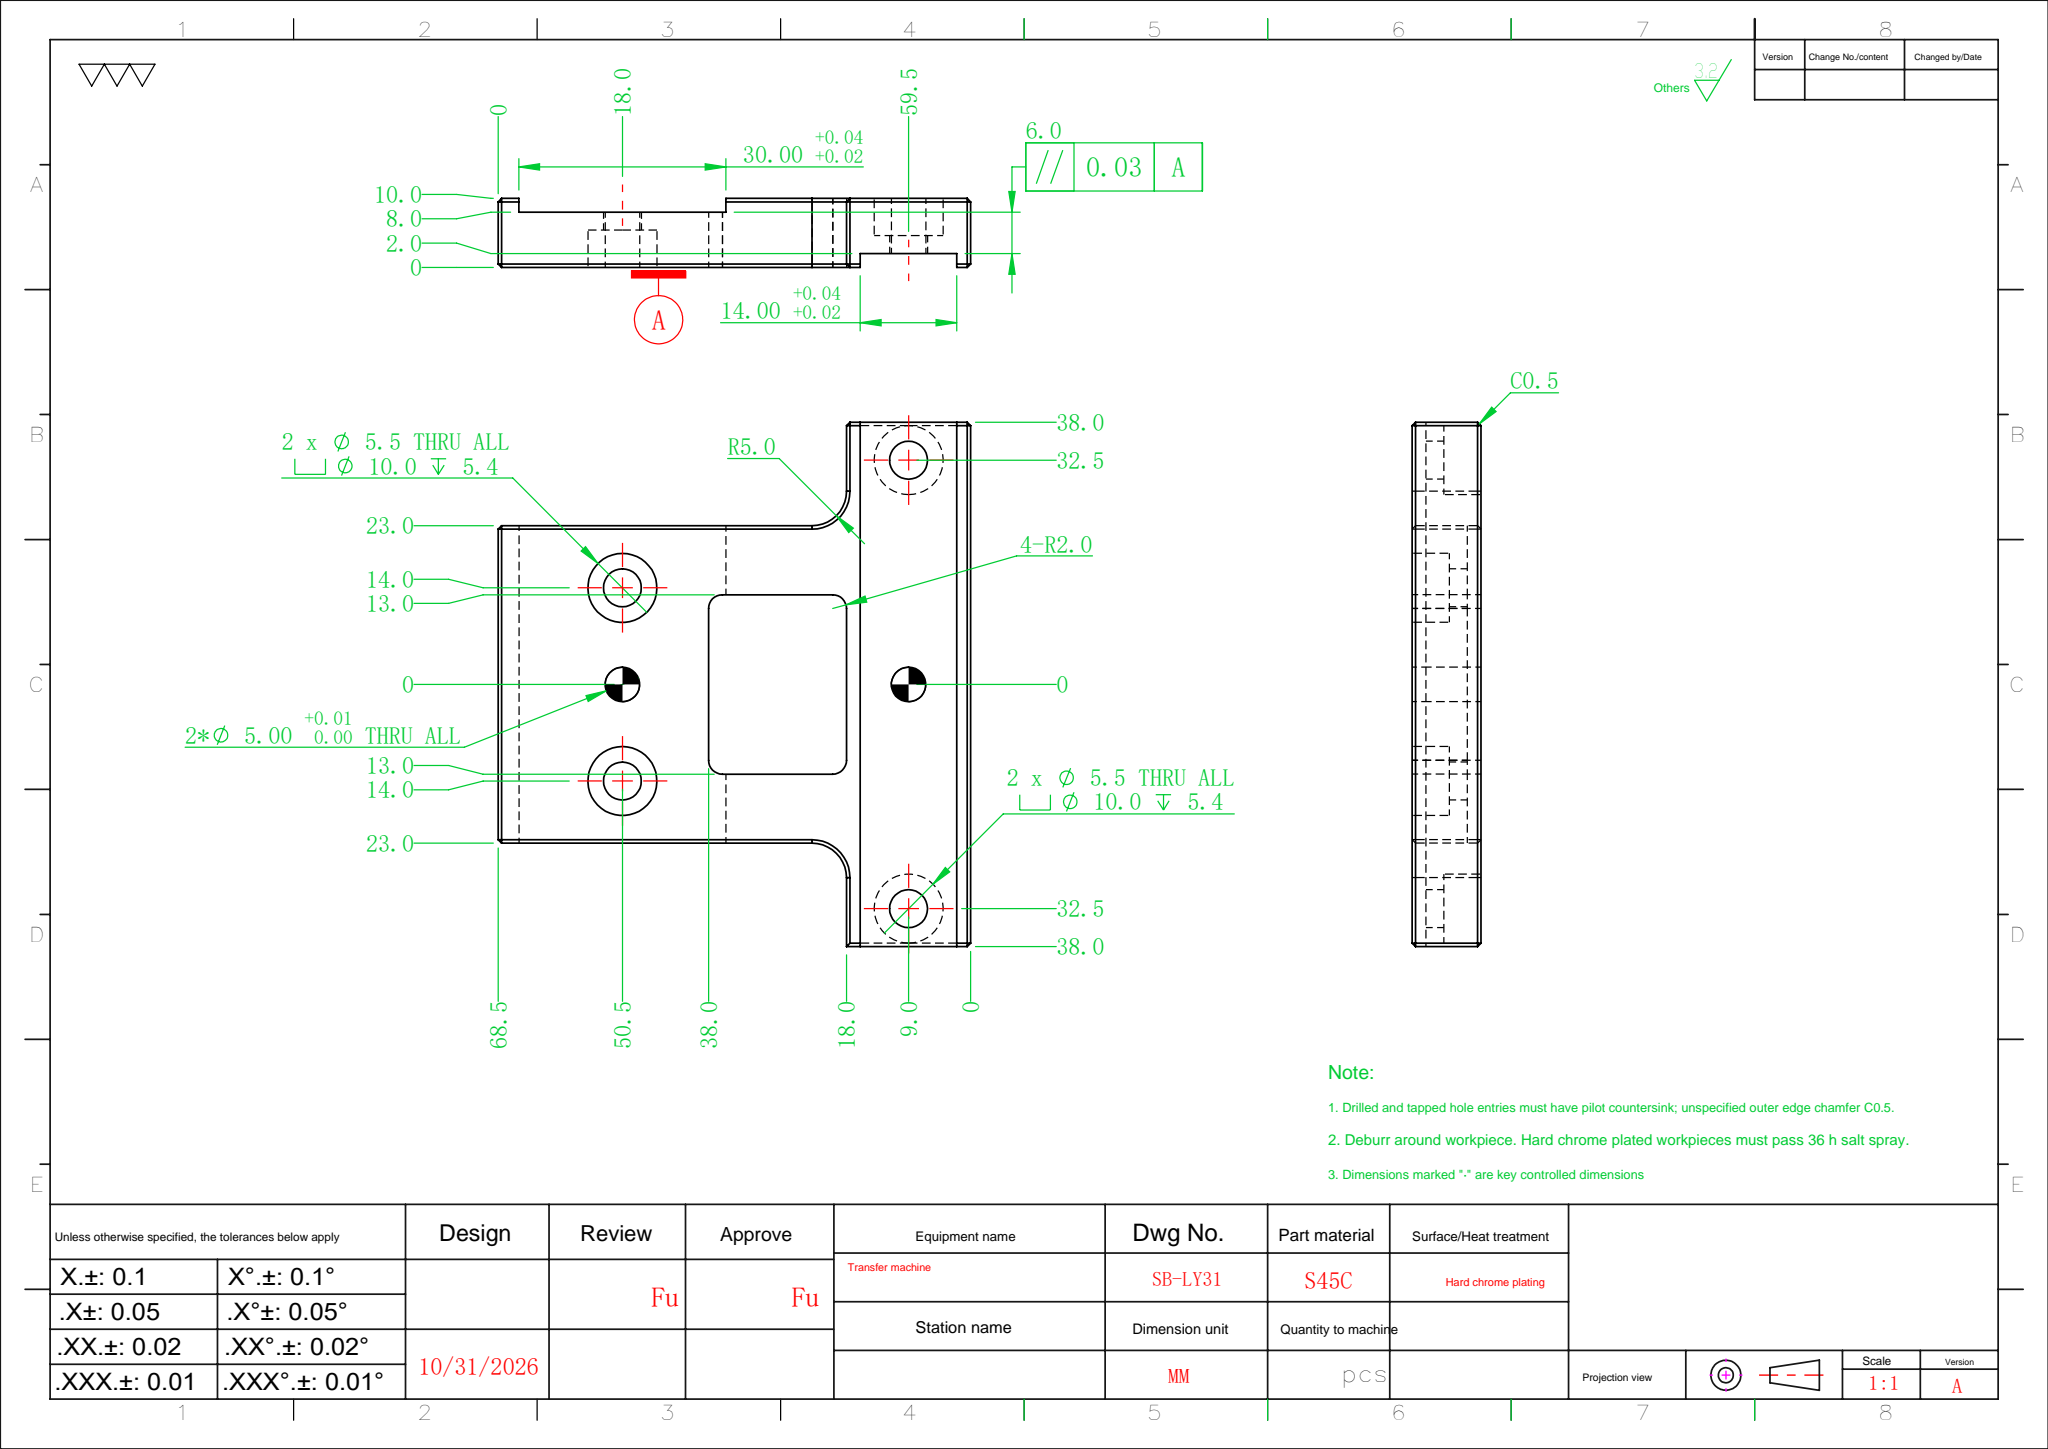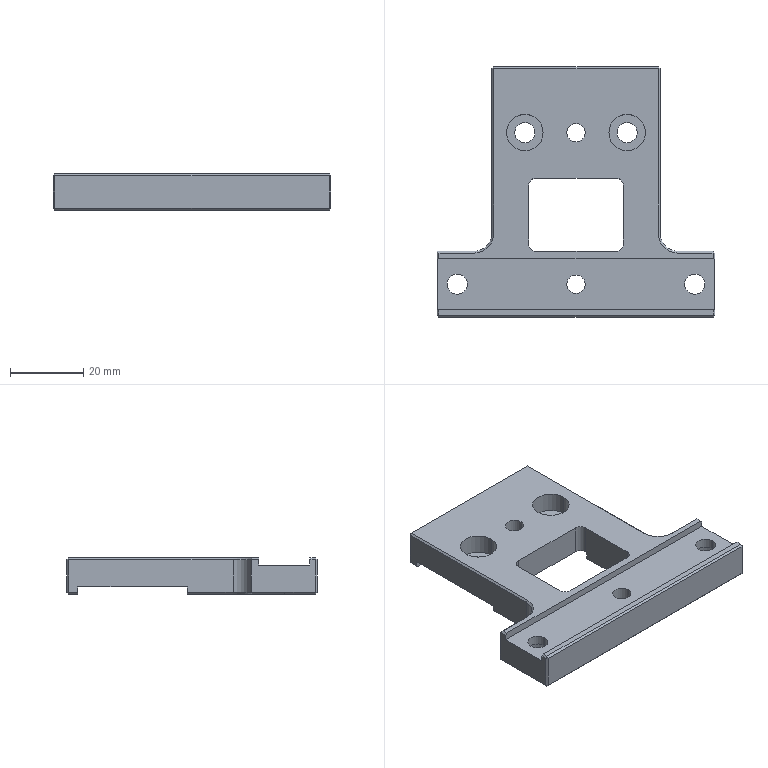Part | SolidWorks | features HoleWzd 4, Cut 3, Fillet 2, Chamfer 1, Extrusion 1, ICE 1 | 1 solid | 92 faces | box 76 x 68.5 x 10 mm | volume 24767 mm3 | plane 62 | cylinder 26 | cone 4 | commonest cylinder face diameters 10 x10 5.5 x8 4 x4 5 x4